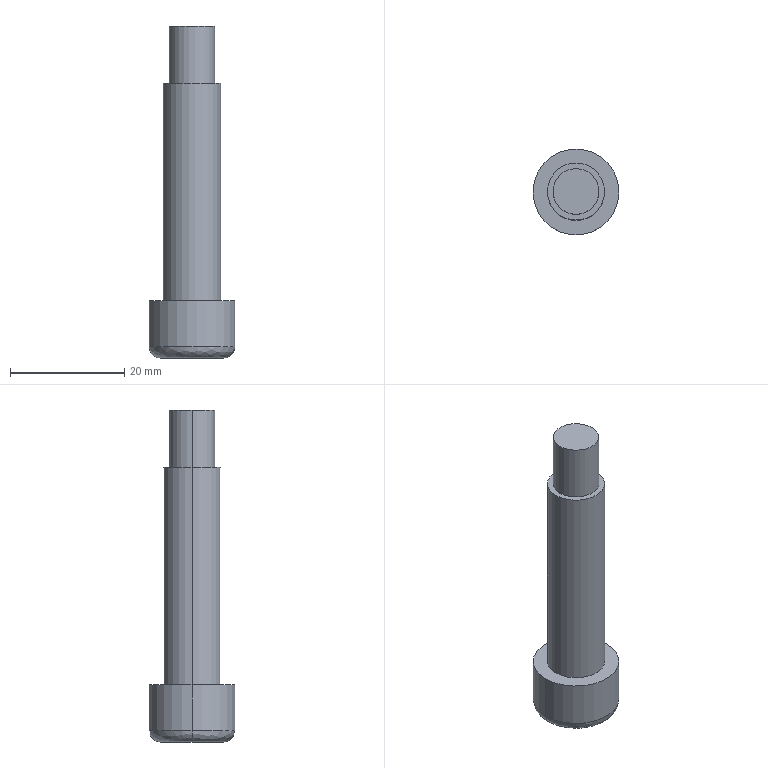Part | STEP file | BULONG BAC M8X10X38 | 1 solid | 19 faces | box 15 x 15 x 58 mm | volume 4939 mm3 | plane 11 | cylinder 6 | spline 2 | commonest cylinder face diameters 8 x2 10 x2 15 x2
STEP:
#1=CARTESIAN_POINT('',(0.,0.,0.));
#2=DIRECTION('',(0.,0.,1.));
#3=DIRECTION('',(1.,0.,0.));
#4=AXIS2_PLACEMENT_3D('',#1,#2,#3);
#5=CARTESIAN_POINT('',(-5.5,0.,0.));
#6=VERTEX_POINT('',#5);
#7=CARTESIAN_POINT('',(5.5,0.,0.));
#8=VERTEX_POINT('',#7);
#9=CARTESIAN_POINT('',(-5.5,0.,0.));
#10=CARTESIAN_POINT('',(-5.5,-11.,0.));
#11=CARTESIAN_POINT('',(5.5,-11.,0.));
#12=CARTESIAN_POINT('',(5.5,0.,0.));
#13=(BOUNDED_CURVE()B_SPLINE_CURVE(3,(#9,#10,#11,#12),.UNSPECIFIED.,.F.,.F.)B_SPLINE_CURVE_WITH_KNOTS((4,4),(0.5,1.),.PIECEWISE_BEZIER_KNOTS.)CURVE()GEOMETRIC_REPRESENTATION_ITEM()RATIONAL_B_SPLINE_CURVE((1.,0.3333,0.3333,1.))REPRESENTATION_ITEM(''));
#14=CARTESIAN_POINT('',(5.5,0.,0.));
#15=CARTESIAN_POINT('',(5.5,-11.,0.));
#16=CARTESIAN_POINT('',(-5.5,-11.,0.));
#17=CARTESIAN_POINT('',(-5.5,0.,0.));
#18=CARTESIAN_POINT('',(6.672,0.,0.));
#19=CARTESIAN_POINT('',(6.672,-13.343,0.));
#20=CARTESIAN_POINT('',(-6.672,-13.343,0.));
#21=CARTESIAN_POINT('',(-6.672,0.,0.));
#22=CARTESIAN_POINT('',(7.5,0.,0.8284));
#23=CARTESIAN_POINT('',(7.5,-15.,0.8284));
#24=CARTESIAN_POINT('',(-7.5,-15.,0.8284));
#25=CARTESIAN_POINT('',(-7.5,0.,0.8284));
#26=CARTESIAN_POINT('',(7.5,0.,2.));
#27=CARTESIAN_POINT('',(7.5,-15.,2.));
#28=CARTESIAN_POINT('',(-7.5,-15.,2.));
#29=CARTESIAN_POINT('',(-7.5,0.,2.));
#30=(BOUNDED_SURFACE()B_SPLINE_SURFACE(3,3,((#14,#15,#16,#17),(#18,#19,#20,#21),(#22,#23,#24,#25),(#26,#27,#28,#29)),.UNSPECIFIED.,.F.,.F.,.F.)B_SPLINE_SURFACE_WITH_KNOTS((4,4),(4,4),(0.,1.),(0.,1.),.PIECEWISE_BEZIER_KNOTS.)GEOMETRIC_REPRESENTATION_ITEM()RATIONAL_B_SPLINE_SURFACE(((1.,0.3333,0.3333,1.),(0.8047,0.2682,0.2682,0.8047),(0.8047,0.2682,0.2682,0.8047),(1.,0.3333,0.3333,1.)))REPRESENTATION_ITEM('')SURFACE());
#31=CARTESIAN_POINT('',(0.,1.));
#32=CARTESIAN_POINT('',(0.,0.));
#33=B_SPLINE_CURVE_WITH_KNOTS('',1,(#31,#32),.UNSPECIFIED.,.F.,.F.,(2,2),(0.5,1.),.PIECEWISE_BEZIER_KNOTS.);
#34=(GEOMETRIC_REPRESENTATION_CONTEXT(2)PARAMETRIC_REPRESENTATION_CONTEXT()REPRESENTATION_CONTEXT('',''));
#35=DEFINITIONAL_REPRESENTATION('',(#33),#34);
#36=PCURVE('',#30,#35);
#37=CARTESIAN_POINT('',(0.,0.,0.));
#38=DIRECTION('',(0.,0.,-1.));
#39=DIRECTION('',(-1.,0.,0.));
#40=AXIS2_PLACEMENT_3D('',#37,#38,#39);
#41=PLANE('',#40);
#42=CARTESIAN_POINT('',(5.5,0.));
#43=CARTESIAN_POINT('',(5.5,-11.));
#44=CARTESIAN_POINT('',(-5.5,-11.));
#45=CARTESIAN_POINT('',(-5.5,0.));
#46=(BOUNDED_CURVE()B_SPLINE_CURVE(3,(#42,#43,#44,#45),.UNSPECIFIED.,.F.,.F.)B_SPLINE_CURVE_WITH_KNOTS((4,4),(0.5,1.),.PIECEWISE_BEZIER_KNOTS.)CURVE()GEOMETRIC_REPRESENTATION_ITEM()RATIONAL_B_SPLINE_CURVE((1.,0.3333,0.3333,1.))REPRESENTATION_ITEM(''));
#47=(GEOMETRIC_REPRESENTATION_CONTEXT(2)PARAMETRIC_REPRESENTATION_CONTEXT()REPRESENTATION_CONTEXT('',''));
#48=DEFINITIONAL_REPRESENTATION('',(#46),#47);
#49=PCURVE('',#41,#48);
#50=SURFACE_CURVE('',#13,(#36,#49),.PCURVE_S1.);
#51=EDGE_CURVE('',#6,#8,#50,.T.);
#52=ORIENTED_EDGE('',*,*,#51,.T.);
#53=CARTESIAN_POINT('',(7.5,0.,2.));
#54=VERTEX_POINT('',#53);
#55=CARTESIAN_POINT('',(5.5,0.,2.));
#56=DIRECTION('',(0.,-1.,0.));
#57=DIRECTION('',(1.,0.,0.));
#58=AXIS2_PLACEMENT_3D('',#55,#56,#57);
#59=CIRCLE('',#58,2.);
#60=CARTESIAN_POINT('',(0.,0.));
#61=CARTESIAN_POINT('',(0.01683,0.));
#62=CARTESIAN_POINT('',(0.04999,0.));
#63=CARTESIAN_POINT('',(0.09843,0.));
#64=CARTESIAN_POINT('',(0.1457,0.));
#65=CARTESIAN_POINT('',(0.192,0.));
#66=CARTESIAN_POINT('',(0.2375,0.));
#67=CARTESIAN_POINT('',(0.2823,0.));
#68=CARTESIAN_POINT('',(0.3265,0.));
#69=CARTESIAN_POINT('',(0.3703,0.));
#70=CARTESIAN_POINT('',(0.4137,0.));
#71=CARTESIAN_POINT('',(0.4569,0.));
#72=CARTESIAN_POINT('',(0.5,0.));
#73=CARTESIAN_POINT('',(0.5431,0.));
#74=CARTESIAN_POINT('',(0.5863,0.));
#75=CARTESIAN_POINT('',(0.6297,0.));
#76=CARTESIAN_POINT('',(0.6735,0.));
#77=CARTESIAN_POINT('',(0.7177,0.));
#78=CARTESIAN_POINT('',(0.7625,0.));
#79=CARTESIAN_POINT('',(0.808,0.));
#80=CARTESIAN_POINT('',(0.8543,0.));
#81=CARTESIAN_POINT('',(0.9016,0.));
#82=CARTESIAN_POINT('',(0.95,0.));
#83=CARTESIAN_POINT('',(0.9832,0.));
#84=CARTESIAN_POINT('',(1.,0.));
#85=B_SPLINE_CURVE_WITH_KNOTS('',3,(#60,#61,#62,#63,#64,#65,#66,#67,#68,#69,#70,#71,#72,#73,#74,#75,#76,#77,#78,#79,#80,#81,#82,#83,#84),.UNSPECIFIED.,.F.,.F.,(4,1,1,1,1,1,1,1,1,1,1,1,1,1,1,1,1,1,1,1,1,1,4),(4.712,4.784,4.855,4.927,4.998,5.069,5.141,5.212,5.284,5.355,5.426,5.498,5.569,5.641,5.712,5.783,5.855,5.926,5.998,6.069,6.14,6.212,6.283),.QUASI_UNIFORM_KNOTS.);
#86=(GEOMETRIC_REPRESENTATION_CONTEXT(2)PARAMETRIC_REPRESENTATION_CONTEXT()REPRESENTATION_CONTEXT('',''));
#87=DEFINITIONAL_REPRESENTATION('',(#85),#86);
#88=PCURVE('',#30,#87);
#89=CARTESIAN_POINT('',(-5.5,0.,0.));
#90=CARTESIAN_POINT('',(-5.5,11.,0.));
#91=CARTESIAN_POINT('',(5.5,11.,0.));
#92=CARTESIAN_POINT('',(5.5,0.,0.));
#93=CARTESIAN_POINT('',(-6.672,0.,0.));
#94=CARTESIAN_POINT('',(-6.672,13.343,0.));
#95=CARTESIAN_POINT('',(6.672,13.343,0.));
#96=CARTESIAN_POINT('',(6.672,0.,0.));
#97=CARTESIAN_POINT('',(-7.5,0.,0.8284));
#98=CARTESIAN_POINT('',(-7.5,15.,0.8284));
#99=CARTESIAN_POINT('',(7.5,15.,0.8284));
#100=CARTESIAN_POINT('',(7.5,0.,0.8284));
#101=CARTESIAN_POINT('',(-7.5,0.,2.));
#102=CARTESIAN_POINT('',(-7.5,15.,2.));
#103=CARTESIAN_POINT('',(7.5,15.,2.));
#104=CARTESIAN_POINT('',(7.5,0.,2.));
#105=(BOUNDED_SURFACE()B_SPLINE_SURFACE(3,3,((#89,#90,#91,#92),(#93,#94,#95,#96),(#97,#98,#99,#100),(#101,#102,#103,#104)),.UNSPECIFIED.,.F.,.F.,.F.)B_SPLINE_SURFACE_WITH_KNOTS((4,4),(4,4),(0.,1.),(0.,1.),.PIECEWISE_BEZIER_KNOTS.)GEOMETRIC_REPRESENTATION_ITEM()RATIONAL_B_SPLINE_SURFACE(((1.,0.3333,0.3333,1.),(0.8047,0.2682,0.2682,0.8047),(0.8047,0.2682,0.2682,0.8047),(1.,0.3333,0.3333,1.)))REPRESENTATION_ITEM('')SURFACE());
#106=CARTESIAN_POINT('',(0.,1.));
#107=CARTESIAN_POINT('',(0.01683,1.));
#108=CARTESIAN_POINT('',(0.04999,1.));
#109=CARTESIAN_POINT('',(0.09843,1.));
#110=CARTESIAN_POINT('',(0.1457,1.));
#111=CARTESIAN_POINT('',(0.192,1.));
#112=CARTESIAN_POINT('',(0.2375,1.));
#113=CARTESIAN_POINT('',(0.2823,1.));
#114=CARTESIAN_POINT('',(0.3265,1.));
#115=CARTESIAN_POINT('',(0.3703,1.));
#116=CARTESIAN_POINT('',(0.4137,1.));
#117=CARTESIAN_POINT('',(0.4569,1.));
#118=CARTESIAN_POINT('',(0.5,1.));
#119=CARTESIAN_POINT('',(0.5431,1.));
#120=CARTESIAN_POINT('',(0.5863,1.));
#121=CARTESIAN_POINT('',(0.6297,1.));
#122=CARTESIAN_POINT('',(0.6735,1.));
#123=CARTESIAN_POINT('',(0.7177,1.));
#124=CARTESIAN_POINT('',(0.7625,1.));
#125=CARTESIAN_POINT('',(0.808,1.));
#126=CARTESIAN_POINT('',(0.8543,1.));
#127=CARTESIAN_POINT('',(0.9016,1.));
#128=CARTESIAN_POINT('',(0.95,1.));
#129=CARTESIAN_POINT('',(0.9832,1.));
#130=CARTESIAN_POINT('',(1.,1.));
#131=B_SPLINE_CURVE_WITH_KNOTS('',3,(#106,#107,#108,#109,#110,#111,#112,#113,#114,#115,#116,#117,#118,#119,#120,#121,#122,#123,#124,#125,#126,#127,#128,#129,#130),.UNSPECIFIED.,.F.,.F.,(4,1,1,1,1,1,1,1,1,1,1,1,1,1,1,1,1,1,1,1,1,1,4),(4.712,4.784,4.855,4.927,4.998,5.069,5.141,5.212,5.284,5.355,5.426,5.498,5.569,5.641,5.712,5.783,5.855,5.926,5.998,6.069,6.14,6.212,6.283),.QUASI_UNIFORM_KNOTS.);
#132=(GEOMETRIC_REPRESENTATION_CONTEXT(2)PARAMETRIC_REPRESENTATION_CONTEXT()REPRESENTATION_CONTEXT('',''));
#133=DEFINITIONAL_REPRESENTATION('',(#131),#132);
#134=PCURVE('',#105,#133);
#135=SURFACE_CURVE('',#59,(#88,#134),.PCURVE_S1.);
#136=EDGE_CURVE('',#8,#54,#135,.T.);
#137=ORIENTED_EDGE('',*,*,#136,.T.);
#138=CARTESIAN_POINT('',(-7.5,0.,2.));
#139=VERTEX_POINT('',#138);
#140=CARTESIAN_POINT('',(0.,0.,2.));
#141=DIRECTION('',(0.,0.,1.));
#142=DIRECTION('',(1.,0.,0.));
#143=AXIS2_PLACEMENT_3D('',#140,#141,#142);
#144=CIRCLE('',#143,7.5);
#145=CARTESIAN_POINT('',(1.,1.));
#146=CARTESIAN_POINT('',(1.,0.9763));
#147=CARTESIAN_POINT('',(1.,0.9319));
#148=CARTESIAN_POINT('',(1.,0.8733));
#149=CARTESIAN_POINT('',(1.,0.8206));
#150=CARTESIAN_POINT('',(1.,0.7724));
#151=CARTESIAN_POINT('',(1.,0.7279));
#152=CARTESIAN_POINT('',(1.,0.6861));
#153=CARTESIAN_POINT('',(1.,0.6465));
#154=CARTESIAN_POINT('',(1.,0.6086));
#155=CARTESIAN_POINT('',(1.,0.5718));
#156=CARTESIAN_POINT('',(1.,0.5357));
#157=CARTESIAN_POINT('',(1.,0.5));
#158=CARTESIAN_POINT('',(1.,0.4643));
#159=CARTESIAN_POINT('',(1.,0.4282));
#160=CARTESIAN_POINT('',(1.,0.3914));
#161=CARTESIAN_POINT('',(1.,0.3535));
#162=CARTESIAN_POINT('',(1.,0.3139));
#163=CARTESIAN_POINT('',(1.,0.2721));
#164=CARTESIAN_POINT('',(1.,0.2276));
#165=CARTESIAN_POINT('',(1.,0.1794));
#166=CARTESIAN_POINT('',(1.,0.1267));
#167=CARTESIAN_POINT('',(1.,0.06805));
#168=CARTESIAN_POINT('',(1.,0.02375));
#169=CARTESIAN_POINT('',(1.,0.));
#170=B_SPLINE_CURVE_WITH_KNOTS('',3,(#145,#146,#147,#148,#149,#150,#151,#152,#153,#154,#155,#156,#157,#158,#159,#160,#161,#162,#163,#164,#165,#166,#167,#168,#169),.UNSPECIFIED.,.F.,.F.,(4,1,1,1,1,1,1,1,1,1,1,1,1,1,1,1,1,1,1,1,1,1,4),(3.142,3.284,3.427,3.57,3.713,3.856,3.998,4.141,4.284,4.427,4.57,4.712,4.855,4.998,5.141,5.284,5.426,5.569,5.712,5.855,5.998,6.14,6.283),.QUASI_UNIFORM_KNOTS.);
#171=(GEOMETRIC_REPRESENTATION_CONTEXT(2)PARAMETRIC_REPRESENTATION_CONTEXT()REPRESENTATION_CONTEXT('',''));
#172=DEFINITIONAL_REPRESENTATION('',(#170),#171);
#173=PCURVE('',#30,#172);
#174=CARTESIAN_POINT('',(0.,0.,0.));
#175=DIRECTION('',(0.,0.,1.));
#176=DIRECTION('',(1.,0.,0.));
#177=AXIS2_PLACEMENT_3D('',#174,#175,#176);
#178=CYLINDRICAL_SURFACE('',#177,7.5);
#179=CARTESIAN_POINT('',(0.,2.));
#180=DIRECTION('',(1.,0.));
#181=VECTOR('',#180,1.);
#182=LINE('',#179,#181);
#183=(GEOMETRIC_REPRESENTATION_CONTEXT(2)PARAMETRIC_REPRESENTATION_CONTEXT()REPRESENTATION_CONTEXT('',''));
#184=DEFINITIONAL_REPRESENTATION('',(#182),#183);
#185=PCURVE('',#178,#184);
#186=SURFACE_CURVE('',#144,(#173,#185),.PCURVE_S1.);
#187=EDGE_CURVE('',#139,#54,#186,.T.);
#188=ORIENTED_EDGE('',*,*,#187,.F.);
#189=CARTESIAN_POINT('',(-5.5,0.,2.));
#190=DIRECTION('',(0.,1.,0.));
#191=DIRECTION('',(-1.,0.,0.));
#192=AXIS2_PLACEMENT_3D('',#189,#190,#191);
#193=CIRCLE('',#192,2.);
#194=CARTESIAN_POINT('',(0.,1.));
#195=CARTESIAN_POINT('',(0.01683,1.));
#196=CARTESIAN_POINT('',(0.04999,1.));
#197=CARTESIAN_POINT('',(0.09843,1.));
#198=CARTESIAN_POINT('',(0.1457,1.));
#199=CARTESIAN_POINT('',(0.192,1.));
#200=CARTESIAN_POINT('',(0.2375,1.));
#201=CARTESIAN_POINT('',(0.2823,1.));
#202=CARTESIAN_POINT('',(0.3265,1.));
#203=CARTESIAN_POINT('',(0.3703,1.));
#204=CARTESIAN_POINT('',(0.4137,1.));
#205=CARTESIAN_POINT('',(0.4569,1.));
#206=CARTESIAN_POINT('',(0.5,1.));
#207=CARTESIAN_POINT('',(0.5431,1.));
#208=CARTESIAN_POINT('',(0.5863,1.));
#209=CARTESIAN_POINT('',(0.6297,1.));
#210=CARTESIAN_POINT('',(0.6735,1.));
#211=CARTESIAN_POINT('',(0.7177,1.));
#212=CARTESIAN_POINT('',(0.7625,1.));
#213=CARTESIAN_POINT('',(0.808,1.));
#214=CARTESIAN_POINT('',(0.8543,1.));
#215=CARTESIAN_POINT('',(0.9016,1.));
#216=CARTESIAN_POINT('',(0.95,1.));
#217=CARTESIAN_POINT('',(0.9832,1.));
#218=CARTESIAN_POINT('',(1.,1.));
#219=B_SPLINE_CURVE_WITH_KNOTS('',3,(#194,#195,#196,#197,#198,#199,#200,#201,#202,#203,#204,#205,#206,#207,#208,#209,#210,#211,#212,#213,#214,#215,#216,#217,#218),.UNSPECIFIED.,.F.,.F.,(4,1,1,1,1,1,1,1,1,1,1,1,1,1,1,1,1,1,1,1,1,1,4),(4.712,4.784,4.855,4.927,4.998,5.069,5.141,5.212,5.284,5.355,5.426,5.498,5.569,5.641,5.712,5.783,5.855,5.926,5.998,6.069,6.14,6.212,6.283),.QUASI_UNIFORM_KNOTS.);
#220=(GEOMETRIC_REPRESENTATION_CONTEXT(2)PARAMETRIC_REPRESENTATION_CONTEXT()REPRESENTATION_CONTEXT('',''));
#221=DEFINITIONAL_REPRESENTATION('',(#219),#220);
#222=PCURVE('',#30,#221);
#223=CARTESIAN_POINT('',(0.,0.));
#224=CARTESIAN_POINT('',(0.01683,0.));
#225=CARTESIAN_POINT('',(0.04999,0.));
#226=CARTESIAN_POINT('',(0.09843,0.));
#227=CARTESIAN_POINT('',(0.1457,0.));
#228=CARTESIAN_POINT('',(0.192,0.));
#229=CARTESIAN_POINT('',(0.2375,0.));
#230=CARTESIAN_POINT('',(0.2823,0.));
#231=CARTESIAN_POINT('',(0.3265,0.));
#232=CARTESIAN_POINT('',(0.3703,0.));
#233=CARTESIAN_POINT('',(0.4137,0.));
#234=CARTESIAN_POINT('',(0.4569,0.));
#235=CARTESIAN_POINT('',(0.5,0.));
#236=CARTESIAN_POINT('',(0.5431,0.));
#237=CARTESIAN_POINT('',(0.5863,0.));
#238=CARTESIAN_POINT('',(0.6297,0.));
#239=CARTESIAN_POINT('',(0.6735,0.));
#240=CARTESIAN_POINT('',(0.7177,0.));
#241=CARTESIAN_POINT('',(0.7625,0.));
#242=CARTESIAN_POINT('',(0.808,0.));
#243=CARTESIAN_POINT('',(0.8543,0.));
#244=CARTESIAN_POINT('',(0.9016,0.));
#245=CARTESIAN_POINT('',(0.95,0.));
#246=CARTESIAN_POINT('',(0.9832,0.));
#247=CARTESIAN_POINT('',(1.,0.));
#248=B_SPLINE_CURVE_WITH_KNOTS('',3,(#223,#224,#225,#226,#227,#228,#229,#230,#231,#232,#233,#234,#235,#236,#237,#238,#239,#240,#241,#242,#243,#244,#245,#246,#247),.UNSPECIFIED.,.F.,.F.,(4,1,1,1,1,1,1,1,1,1,1,1,1,1,1,1,1,1,1,1,1,1,4),(4.712,4.784,4.855,4.927,4.998,5.069,5.141,5.212,5.284,5.355,5.426,5.498,5.569,5.641,5.712,5.783,5.855,5.926,5.998,6.069,6.14,6.212,6.283),.QUASI_UNIFORM_KNOTS.);
#249=(GEOMETRIC_REPRESENTATION_CONTEXT(2)PARAMETRIC_REPRESENTATION_CONTEXT()REPRESENTATION_CONTEXT('',''));
#250=DEFINITIONAL_REPRESENTATION('',(#248),#249);
#251=PCURVE('',#105,#250);
#252=SURFACE_CURVE('',#193,(#222,#251),.PCURVE_S1.);
#253=EDGE_CURVE('',#6,#139,#252,.T.);
#254=ORIENTED_EDGE('',*,*,#253,.F.);
#255=EDGE_LOOP('',(#52,#137,#188,#254));
#256=FACE_BOUND('',#255,.T.);
#257=ADVANCED_FACE('',(#256),#30,.T.);
#258=CARTESIAN_POINT('',(5.,0.,10.));
#259=VERTEX_POINT('',#258);
#260=CARTESIAN_POINT('',(-5.,0.,10.));
#261=VERTEX_POINT('',#260);
#262=CARTESIAN_POINT('',(0.,0.,10.));
#263=DIRECTION('',(0.,0.,1.));
#264=DIRECTION('',(1.,0.,0.));
#265=AXIS2_PLACEMENT_3D('',#262,#263,#264);
#266=CIRCLE('',#265,5.);
#267=CARTESIAN_POINT('',(0.,0.,10.));
#268=DIRECTION('',(0.,0.,1.));
#269=DIRECTION('',(1.,0.,0.));
#270=AXIS2_PLACEMENT_3D('',#267,#268,#269);
#271=CYLINDRICAL_SURFACE('',#270,5.);
#272=CARTESIAN_POINT('',(0.,0.));
#273=DIRECTION('',(1.,0.));
#274=VECTOR('',#273,1.);
#275=LINE('',#272,#274);
#276=(GEOMETRIC_REPRESENTATION_CONTEXT(2)PARAMETRIC_REPRESENTATION_CONTEXT()REPRESENTATION_CONTEXT('',''));
#277=DEFINITIONAL_REPRESENTATION('',(#275),#276);
#278=PCURVE('',#271,#277);
#279=CARTESIAN_POINT('',(0.,0.,10.));
#280=DIRECTION('',(0.,0.,-1.));
#281=DIRECTION('',(-1.,0.,0.));
#282=AXIS2_PLACEMENT_3D('',#279,#280,#281);
#283=PLANE('',#282);
#284=CARTESIAN_POINT('',(-5.,0.));
#285=CARTESIAN_POINT('',(-5.,8.66));
#286=CARTESIAN_POINT('',(2.5,4.33));
#287=CARTESIAN_POINT('',(10.,0.));
#288=CARTESIAN_POINT('',(2.5,-4.33));
#289=CARTESIAN_POINT('',(-5.,-8.66));
#290=CARTESIAN_POINT('',(-5.,0.));
#291=(BOUNDED_CURVE()B_SPLINE_CURVE(2,(#284,#285,#286,#287,#288,#289,#290),.UNSPECIFIED.,.T.,.F.)B_SPLINE_CURVE_WITH_KNOTS((1,2,2,2,2,1),(-2.094,0.,2.094,4.189,6.283,8.378),.UNSPECIFIED.)CURVE()GEOMETRIC_REPRESENTATION_ITEM()RATIONAL_B_SPLINE_CURVE((1.,0.5,1.,0.5,1.,0.5,1.))REPRESENTATION_ITEM(''));
#292=(GEOMETRIC_REPRESENTATION_CONTEXT(2)PARAMETRIC_REPRESENTATION_CONTEXT()REPRESENTATION_CONTEXT('',''));
#293=DEFINITIONAL_REPRESENTATION('',(#291),#292);
#294=PCURVE('',#283,#293);
#295=SURFACE_CURVE('',#266,(#278,#294),.PCURVE_S1.);
#296=EDGE_CURVE('',#259,#261,#295,.T.);
#297=ORIENTED_EDGE('',*,*,#296,.T.);
#298=CARTESIAN_POINT('',(-5.,0.,48.));
#299=VERTEX_POINT('',#298);
#300=CARTESIAN_POINT('',(-5.,0.,10.));
#301=DIRECTION('',(0.,0.,1.));
#302=VECTOR('',#301,1.);
#303=LINE('',#300,#302);
#304=CARTESIAN_POINT('',(3.142,0.));
#305=DIRECTION('',(0.,1.));
#306=VECTOR('',#305,1.);
#307=LINE('',#304,#306);
#308=(GEOMETRIC_REPRESENTATION_CONTEXT(2)PARAMETRIC_REPRESENTATION_CONTEXT()REPRESENTATION_CONTEXT('',''));
#309=DEFINITIONAL_REPRESENTATION('',(#307),#308);
#310=PCURVE('',#271,#309);
#311=CARTESIAN_POINT('',(0.,0.,10.));
#312=DIRECTION('',(0.,0.,1.));
#313=DIRECTION('',(1.,0.,0.));
#314=AXIS2_PLACEMENT_3D('',#311,#312,#313);
#315=CYLINDRICAL_SURFACE('',#314,5.);
#316=CARTESIAN_POINT('',(3.142,0.));
#317=DIRECTION('',(0.,1.));
#318=VECTOR('',#317,1.);
#319=LINE('',#316,#318);
#320=(GEOMETRIC_REPRESENTATION_CONTEXT(2)PARAMETRIC_REPRESENTATION_CONTEXT()REPRESENTATION_CONTEXT('',''));
#321=DEFINITIONAL_REPRESENTATION('',(#319),#320);
#322=PCURVE('',#315,#321);
#323=SURFACE_CURVE('',#303,(#310,#322),.PCURVE_S1.);
#324=EDGE_CURVE('',#261,#299,#323,.T.);
#325=ORIENTED_EDGE('',*,*,#324,.T.);
#326=CARTESIAN_POINT('',(5.,0.,48.));
#327=VERTEX_POINT('',#326);
#328=CARTESIAN_POINT('',(0.,0.,48.));
#329=DIRECTION('',(0.,0.,-1.));
#330=DIRECTION('',(1.,0.,0.));
#331=AXIS2_PLACEMENT_3D('',#328,#329,#330);
#332=CIRCLE('',#331,5.);
#333=CARTESIAN_POINT('',(6.283,38.));
#334=DIRECTION('',(-1.,0.));
#335=VECTOR('',#334,1.);
#336=LINE('',#333,#335);
#337=(GEOMETRIC_REPRESENTATION_CONTEXT(2)PARAMETRIC_REPRESENTATION_CONTEXT()REPRESENTATION_CONTEXT('',''));
#338=DEFINITIONAL_REPRESENTATION('',(#336),#337);
#339=PCURVE('',#271,#338);
#340=CARTESIAN_POINT('',(0.,0.,48.));
#341=DIRECTION('',(0.,0.,-1.));
#342=DIRECTION('',(-1.,0.,0.));
#343=AXIS2_PLACEMENT_3D('',#340,#341,#342);
#344=PLANE('',#343);
#345=CARTESIAN_POINT('',(0.,0.));
#346=DIRECTION('',(-1.,0.));
#347=AXIS2_PLACEMENT_2D('',#345,#346);
#348=CIRCLE('',#347,5.);
#349=(GEOMETRIC_REPRESENTATION_CONTEXT(2)PARAMETRIC_REPRESENTATION_CONTEXT()REPRESENTATION_CONTEXT('',''));
#350=DEFINITIONAL_REPRESENTATION('',(#348),#349);
#351=PCURVE('',#344,#350);
#352=SURFACE_CURVE('',#332,(#339,#351),.PCURVE_S1.);
#353=EDGE_CURVE('',#299,#327,#352,.T.);
#354=ORIENTED_EDGE('',*,*,#353,.T.);
#355=CARTESIAN_POINT('',(5.,0.,10.));
#356=DIRECTION('',(0.,0.,1.));
#357=VECTOR('',#356,1.);
#358=LINE('',#355,#357);
#359=CARTESIAN_POINT('',(0.,0.));
#360=DIRECTION('',(0.,1.));
#361=VECTOR('',#360,1.);
#362=LINE('',#359,#361);
#363=(GEOMETRIC_REPRESENTATION_CONTEXT(2)PARAMETRIC_REPRESENTATION_CONTEXT()REPRESENTATION_CONTEXT('',''));
#364=DEFINITIONAL_REPRESENTATION('',(#362),#363);
#365=PCURVE('',#271,#364);
#366=CARTESIAN_POINT('',(6.283,0.));
#367=DIRECTION('',(0.,1.));
#368=VECTOR('',#367,1.);
#369=LINE('',#366,#368);
#370=(GEOMETRIC_REPRESENTATION_CONTEXT(2)PARAMETRIC_REPRESENTATION_CONTEXT()REPRESENTATION_CONTEXT('',''));
#371=DEFINITIONAL_REPRESENTATION('',(#369),#370);
#372=PCURVE('',#315,#371);
#373=SURFACE_CURVE('',#358,(#365,#372),.PCURVE_S1.);
#374=EDGE_CURVE('',#259,#327,#373,.T.);
#375=ORIENTED_EDGE('',*,*,#374,.F.);
#376=EDGE_LOOP('',(#297,#325,#354,#375));
#377=FACE_BOUND('',#376,.T.);
#378=ADVANCED_FACE('',(#377),#271,.T.);
#379=CARTESIAN_POINT('',(0.,0.,2.));
#380=DIRECTION('',(0.,0.,1.));
#381=DIRECTION('',(1.,0.,0.));
#382=AXIS2_PLACEMENT_3D('',#379,#380,#381);
#383=CIRCLE('',#382,7.5);
#384=CARTESIAN_POINT('',(0.,0.,0.));
#385=DIRECTION('',(0.,0.,1.));
#386=DIRECTION('',(1.,0.,0.));
#387=AXIS2_PLACEMENT_3D('',#384,#385,#386);
#388=CYLINDRICAL_SURFACE('',#387,7.5);
#389=CARTESIAN_POINT('',(0.,2.));
#390=DIRECTION('',(1.,0.));
#391=VECTOR('',#390,1.);
#392=LINE('',#389,#391);
#393=(GEOMETRIC_REPRESENTATION_CONTEXT(2)PARAMETRIC_REPRESENTATION_CONTEXT()REPRESENTATION_CONTEXT('',''));
#394=DEFINITIONAL_REPRESENTATION('',(#392),#393);
#395=PCURVE('',#388,#394);
#396=CARTESIAN_POINT('',(1.,1.));
#397=CARTESIAN_POINT('',(1.,0.9763));
#398=CARTESIAN_POINT('',(1.,0.9319));
#399=CARTESIAN_POINT('',(1.,0.8733));
#400=CARTESIAN_POINT('',(1.,0.8206));
#401=CARTESIAN_POINT('',(1.,0.7724));
#402=CARTESIAN_POINT('',(1.,0.7279));
#403=CARTESIAN_POINT('',(1.,0.6861));
#404=CARTESIAN_POINT('',(1.,0.6465));
#405=CARTESIAN_POINT('',(1.,0.6086));
#406=CARTESIAN_POINT('',(1.,0.5718));
#407=CARTESIAN_POINT('',(1.,0.5357));
#408=CARTESIAN_POINT('',(1.,0.5));
#409=CARTESIAN_POINT('',(1.,0.4643));
#410=CARTESIAN_POINT('',(1.,0.4282));
#411=CARTESIAN_POINT('',(1.,0.3914));
#412=CARTESIAN_POINT('',(1.,0.3535));
#413=CARTESIAN_POINT('',(1.,0.3139));
#414=CARTESIAN_POINT('',(1.,0.2721));
#415=CARTESIAN_POINT('',(1.,0.2276));
#416=CARTESIAN_POINT('',(1.,0.1794));
#417=CARTESIAN_POINT('',(1.,0.1267));
#418=CARTESIAN_POINT('',(1.,0.06805));
#419=CARTESIAN_POINT('',(1.,0.02375));
#420=CARTESIAN_POINT('',(1.,0.));
#421=B_SPLINE_CURVE_WITH_KNOTS('',3,(#396,#397,#398,#399,#400,#401,#402,#403,#404,#405,#406,#407,#408,#409,#410,#411,#412,#413,#414,#415,#416,#417,#418,#419,#420),.UNSPECIFIED.,.F.,.F.,(4,1,1,1,1,1,1,1,1,1,1,1,1,1,1,1,1,1,1,1,1,1,4),(0.,0.1428,0.2856,0.4284,0.5712,0.714,0.8568,0.9996,1.142,1.285,1.428,1.571,1.714,1.856,1.999,2.142,2.285,2.428,2.57,2.713,2.856,2.999,3.142),.QUASI_UNIFORM_KNOTS.);
#422=(GEOMETRIC_REPRESENTATION_CONTEXT(2)PARAMETRIC_REPRESENTATION_CONTEXT()REPRESENTATION_CONTEXT('',''));
#423=DEFINITIONAL_REPRESENTATION('',(#421),#422);
#424=PCURVE('',#105,#423);
#425=SURFACE_CURVE('',#383,(#395,#424),.PCURVE_S1.);
#426=EDGE_CURVE('',#54,#139,#425,.T.);
#427=ORIENTED_EDGE('',*,*,#426,.T.);
#428=CARTESIAN_POINT('',(-7.5,0.,10.));
#429=VERTEX_POINT('',#428);
#430=CARTESIAN_POINT('',(-7.5,0.,0.));
#431=DIRECTION('',(0.,0.,1.));
#432=VECTOR('',#431,1.);
#433=LINE('',#430,#432);
#434=CARTESIAN_POINT('',(3.142,0.));
#435=DIRECTION('',(0.,1.));
#436=VECTOR('',#435,1.);
#437=LINE('',#434,#436);
#438=(GEOMETRIC_REPRESENTATION_CONTEXT(2)PARAMETRIC_REPRESENTATION_CONTEXT()REPRESENTATION_CONTEXT('',''));
#439=DEFINITIONAL_REPRESENTATION('',(#437),#438);
#440=PCURVE('',#388,#439);
#441=CARTESIAN_POINT('',(3.142,0.));
#442=DIRECTION('',(0.,1.));
#443=VECTOR('',#442,1.);
#444=LINE('',#441,#443);
#445=(GEOMETRIC_REPRESENTATION_CONTEXT(2)PARAMETRIC_REPRESENTATION_CONTEXT()REPRESENTATION_CONTEXT('',''));
#446=DEFINITIONAL_REPRESENTATION('',(#444),#445);
#447=PCURVE('',#178,#446);
#448=SURFACE_CURVE('',#433,(#440,#447),.PCURVE_S1.);
#449=EDGE_CURVE('',#139,#429,#448,.T.);
#450=ORIENTED_EDGE('',*,*,#449,.T.);
#451=CARTESIAN_POINT('',(7.5,0.,10.));
#452=VERTEX_POINT('',#451);
#453=CARTESIAN_POINT('',(0.,0.,10.));
#454=DIRECTION('',(0.,0.,-1.));
#455=DIRECTION('',(1.,0.,0.));
#456=AXIS2_PLACEMENT_3D('',#453,#454,#455);
#457=CIRCLE('',#456,7.5);
#458=CARTESIAN_POINT('',(6.283,10.));
#459=DIRECTION('',(-1.,0.));
#460=VECTOR('',#459,1.);
#461=LINE('',#458,#460);
#462=(GEOMETRIC_REPRESENTATION_CONTEXT(2)PARAMETRIC_REPRESENTATION_CONTEXT()REPRESENTATION_CONTEXT('',''));
#463=DEFINITIONAL_REPRESENTATION('',(#461),#462);
#464=PCURVE('',#388,#463);
#465=CARTESIAN_POINT('',(0.,0.));
#466=DIRECTION('',(-1.,0.));
#467=AXIS2_PLACEMENT_2D('',#465,#466);
#468=CIRCLE('',#467,7.5);
#469=(GEOMETRIC_REPRESENTATION_CONTEXT(2)PARAMETRIC_REPRESENTATION_CONTEXT()REPRESENTATION_CONTEXT('',''));
#470=DEFINITIONAL_REPRESENTATION('',(#468),#469);
#471=PCURVE('',#283,#470);
#472=SURFACE_CURVE('',#457,(#464,#471),.PCURVE_S1.);
#473=EDGE_CURVE('',#429,#452,#472,.T.);
#474=ORIENTED_EDGE('',*,*,#473,.T.);
#475=CARTESIAN_POINT('',(7.5,0.,0.));
#476=DIRECTION('',(0.,0.,1.));
#477=VECTOR('',#476,1.);
#478=LINE('',#475,#477);
#479=CARTESIAN_POINT('',(0.,0.));
#480=DIRECTION('',(0.,1.));
#481=VECTOR('',#480,1.);
#482=LINE('',#479,#481);
#483=(GEOMETRIC_REPRESENTATION_CONTEXT(2)PARAMETRIC_REPRESENTATION_CONTEXT()REPRESENTATION_CONTEXT('',''));
#484=DEFINITIONAL_REPRESENTATION('',(#482),#483);
#485=PCURVE('',#388,#484);
#486=CARTESIAN_POINT('',(6.283,0.));
#487=DIRECTION('',(0.,1.));
#488=VECTOR('',#487,1.);
#489=LINE('',#486,#488);
#490=(GEOMETRIC_REPRESENTATION_CONTEXT(2)PARAMETRIC_REPRESENTATION_CONTEXT()REPRESENTATION_CONTEXT('',''));
#491=DEFINITIONAL_REPRESENTATION('',(#489),#490);
#492=PCURVE('',#178,#491);
#493=SURFACE_CURVE('',#478,(#485,#492),.PCURVE_S1.);
#494=EDGE_CURVE('',#54,#452,#493,.T.);
#495=ORIENTED_EDGE('',*,*,#494,.F.);
#496=EDGE_LOOP('',(#427,#450,#474,#495));
#497=FACE_BOUND('',#496,.T.);
#498=ADVANCED_FACE('',(#497),#388,.T.);
#499=CARTESIAN_POINT('',(4.,0.,48.));
#500=VERTEX_POINT('',#499);
#501=CARTESIAN_POINT('',(-4.,0.,48.));
#502=VERTEX_POINT('',#501);
#503=CARTESIAN_POINT('',(0.,0.,48.));
#504=DIRECTION('',(0.,0.,1.));
#505=DIRECTION('',(1.,0.,0.));
#506=AXIS2_PLACEMENT_3D('',#503,#504,#505);
#507=CIRCLE('',#506,4.);
#508=CARTESIAN_POINT('',(0.,0.,48.));
#509=DIRECTION('',(0.,0.,1.));
#510=DIRECTION('',(1.,0.,0.));
#511=AXIS2_PLACEMENT_3D('',#508,#509,#510);
#512=CYLINDRICAL_SURFACE('',#511,4.);
#513=CARTESIAN_POINT('',(0.,0.));
#514=DIRECTION('',(1.,0.));
#515=VECTOR('',#514,1.);
#516=LINE('',#513,#515);
#517=(GEOMETRIC_REPRESENTATION_CONTEXT(2)PARAMETRIC_REPRESENTATION_CONTEXT()REPRESENTATION_CONTEXT('',''));
#518=DEFINITIONAL_REPRESENTATION('',(#516),#517);
#519=PCURVE('',#512,#518);
#520=CARTESIAN_POINT('',(-4.,0.));
#521=CARTESIAN_POINT('',(-4.,6.928));
#522=CARTESIAN_POINT('',(2.,3.464));
#523=CARTESIAN_POINT('',(8.,0.));
#524=CARTESIAN_POINT('',(2.,-3.464));
#525=CARTESIAN_POINT('',(-4.,-6.928));
#526=CARTESIAN_POINT('',(-4.,0.));
#527=(BOUNDED_CURVE()B_SPLINE_CURVE(2,(#520,#521,#522,#523,#524,#525,#526),.UNSPECIFIED.,.T.,.F.)B_SPLINE_CURVE_WITH_KNOTS((1,2,2,2,2,1),(-2.094,0.,2.094,4.189,6.283,8.378),.UNSPECIFIED.)CURVE()GEOMETRIC_REPRESENTATION_ITEM()RATIONAL_B_SPLINE_CURVE((1.,0.5,1.,0.5,1.,0.5,1.))REPRESENTATION_ITEM(''));
#528=(GEOMETRIC_REPRESENTATION_CONTEXT(2)PARAMETRIC_REPRESENTATION_CONTEXT()REPRESENTATION_CONTEXT('',''));
#529=DEFINITIONAL_REPRESENTATION('',(#527),#528);
#530=PCURVE('',#344,#529);
#531=SURFACE_CURVE('',#507,(#519,#530),.PCURVE_S1.);
#532=EDGE_CURVE('',#500,#502,#531,.T.);
#533=ORIENTED_EDGE('',*,*,#532,.T.);
#534=CARTESIAN_POINT('',(-4.,0.,58.));
#535=VERTEX_POINT('',#534);
#536=CARTESIAN_POINT('',(-4.,0.,48.));
#537=DIRECTION('',(0.,0.,1.));
#538=VECTOR('',#537,1.);
#539=LINE('',#536,#538);
#540=CARTESIAN_POINT('',(3.142,0.));
#541=DIRECTION('',(0.,1.));
#542=VECTOR('',#541,1.);
#543=LINE('',#540,#542);
#544=(GEOMETRIC_REPRESENTATION_CONTEXT(2)PARAMETRIC_REPRESENTATION_CONTEXT()REPRESENTATION_CONTEXT('',''));
#545=DEFINITIONAL_REPRESENTATION('',(#543),#544);
#546=PCURVE('',#512,#545);
#547=CARTESIAN_POINT('',(0.,0.,48.));
#548=DIRECTION('',(0.,0.,1.));
#549=DIRECTION('',(1.,0.,0.));
#550=AXIS2_PLACEMENT_3D('',#547,#548,#549);
#551=CYLINDRICAL_SURFACE('',#550,4.);
#552=CARTESIAN_POINT('',(3.142,0.));
#553=DIRECTION('',(0.,1.));
#554=VECTOR('',#553,1.);
#555=LINE('',#552,#554);
#556=(GEOMETRIC_REPRESENTATION_CONTEXT(2)PARAMETRIC_REPRESENTATION_CONTEXT()REPRESENTATION_CONTEXT('',''));
#557=DEFINITIONAL_REPRESENTATION('',(#555),#556);
#558=PCURVE('',#551,#557);
#559=SURFACE_CURVE('',#539,(#546,#558),.PCURVE_S1.);
#560=EDGE_CURVE('',#502,#535,#559,.T.);
#561=ORIENTED_EDGE('',*,*,#560,.T.);
#562=CARTESIAN_POINT('',(4.,0.,58.));
#563=VERTEX_POINT('',#562);
#564=CARTESIAN_POINT('',(0.,0.,58.));
#565=DIRECTION('',(0.,0.,-1.));
#566=DIRECTION('',(1.,0.,0.));
#567=AXIS2_PLACEMENT_3D('',#564,#565,#566);
#568=CIRCLE('',#567,4.);
#569=CARTESIAN_POINT('',(6.283,10.));
#570=DIRECTION('',(-1.,0.));
#571=VECTOR('',#570,1.);
#572=LINE('',#569,#571);
#573=(GEOMETRIC_REPRESENTATION_CONTEXT(2)PARAMETRIC_REPRESENTATION_CONTEXT()REPRESENTATION_CONTEXT('',''));
#574=DEFINITIONAL_REPRESENTATION('',(#572),#573);
#575=PCURVE('',#512,#574);
#576=CARTESIAN_POINT('',(0.,0.,58.));
#577=DIRECTION('',(0.,0.,-1.));
#578=DIRECTION('',(-1.,0.,0.));
#579=AXIS2_PLACEMENT_3D('',#576,#577,#578);
#580=PLANE('',#579);
#581=CARTESIAN_POINT('',(0.,0.));
#582=DIRECTION('',(-1.,0.));
#583=AXIS2_PLACEMENT_2D('',#581,#582);
#584=CIRCLE('',#583,4.);
#585=(GEOMETRIC_REPRESENTATION_CONTEXT(2)PARAMETRIC_REPRESENTATION_CONTEXT()REPRESENTATION_CONTEXT('',''));
#586=DEFINITIONAL_REPRESENTATION('',(#584),#585);
#587=PCURVE('',#580,#586);
#588=SURFACE_CURVE('',#568,(#575,#587),.PCURVE_S1.);
#589=EDGE_CURVE('',#535,#563,#588,.T.);
#590=ORIENTED_EDGE('',*,*,#589,.T.);
#591=CARTESIAN_POINT('',(4.,0.,48.));
#592=DIRECTION('',(0.,0.,1.));
#593=VECTOR('',#592,1.);
#594=LINE('',#591,#593);
#595=CARTESIAN_POINT('',(0.,0.));
#596=DIRECTION('',(0.,1.));
#597=VECTOR('',#596,1.);
#598=LINE('',#595,#597);
#599=(GEOMETRIC_REPRESENTATION_CONTEXT(2)PARAMETRIC_REPRESENTATION_CONTEXT()REPRESENTATION_CONTEXT('',''));
#600=DEFINITIONAL_REPRESENTATION('',(#598),#599);
#601=PCURVE('',#512,#600);
#602=CARTESIAN_POINT('',(6.283,0.));
#603=DIRECTION('',(0.,1.));
#604=VECTOR('',#603,1.);
#605=LINE('',#602,#604);
#606=(GEOMETRIC_REPRESENTATION_CONTEXT(2)PARAMETRIC_REPRESENTATION_CONTEXT()REPRESENTATION_CONTEXT('',''));
#607=DEFINITIONAL_REPRESENTATION('',(#605),#606);
#608=PCURVE('',#551,#607);
#609=SURFACE_CURVE('',#594,(#601,#608),.PCURVE_S1.);
#610=EDGE_CURVE('',#500,#563,#609,.T.);
#611=ORIENTED_EDGE('',*,*,#610,.F.);
#612=EDGE_LOOP('',(#533,#561,#590,#611));
#613=FACE_BOUND('',#612,.T.);
#614=ADVANCED_FACE('',(#613),#512,.T.);
#615=ORIENTED_EDGE('',*,*,#324,.F.);
#616=CARTESIAN_POINT('',(0.,0.,10.));
#617=DIRECTION('',(0.,0.,1.));
#618=DIRECTION('',(1.,0.,0.));
#619=AXIS2_PLACEMENT_3D('',#616,#617,#618);
#620=CIRCLE('',#619,5.);
#621=CARTESIAN_POINT('',(0.,0.));
#622=DIRECTION('',(1.,0.));
#623=VECTOR('',#622,1.);
#624=LINE('',#621,#623);
#625=(GEOMETRIC_REPRESENTATION_CONTEXT(2)PARAMETRIC_REPRESENTATION_CONTEXT()REPRESENTATION_CONTEXT('',''));
#626=DEFINITIONAL_REPRESENTATION('',(#624),#625);
#627=PCURVE('',#315,#626);
#628=CARTESIAN_POINT('',(-5.,0.));
#629=CARTESIAN_POINT('',(-5.,8.66));
#630=CARTESIAN_POINT('',(2.5,4.33));
#631=CARTESIAN_POINT('',(10.,0.));
#632=CARTESIAN_POINT('',(2.5,-4.33));
#633=CARTESIAN_POINT('',(-5.,-8.66));
#634=CARTESIAN_POINT('',(-5.,0.));
#635=(BOUNDED_CURVE()B_SPLINE_CURVE(2,(#628,#629,#630,#631,#632,#633,#634),.UNSPECIFIED.,.T.,.F.)B_SPLINE_CURVE_WITH_KNOTS((1,2,2,2,2,1),(-2.094,0.,2.094,4.189,6.283,8.378),.UNSPECIFIED.)CURVE()GEOMETRIC_REPRESENTATION_ITEM()RATIONAL_B_SPLINE_CURVE((1.,0.5,1.,0.5,1.,0.5,1.))REPRESENTATION_ITEM(''));
#636=(GEOMETRIC_REPRESENTATION_CONTEXT(2)PARAMETRIC_REPRESENTATION_CONTEXT()REPRESENTATION_CONTEXT('',''));
#637=DEFINITIONAL_REPRESENTATION('',(#635),#636);
#638=PCURVE('',#283,#637);
#639=SURFACE_CURVE('',#620,(#627,#638),.PCURVE_S1.);
#640=EDGE_CURVE('',#261,#259,#639,.T.);
#641=ORIENTED_EDGE('',*,*,#640,.T.);
#642=ORIENTED_EDGE('',*,*,#374,.T.);
#643=CARTESIAN_POINT('',(0.,0.,48.));
#644=DIRECTION('',(0.,0.,-1.));
#645=DIRECTION('',(1.,0.,0.));
#646=AXIS2_PLACEMENT_3D('',#643,#644,#645);
#647=CIRCLE('',#646,5.);
#648=CARTESIAN_POINT('',(6.283,38.));
#649=DIRECTION('',(-1.,0.));
#650=VECTOR('',#649,1.);
#651=LINE('',#648,#650);
#652=(GEOMETRIC_REPRESENTATION_CONTEXT(2)PARAMETRIC_REPRESENTATION_CONTEXT()REPRESENTATION_CONTEXT('',''));
#653=DEFINITIONAL_REPRESENTATION('',(#651),#652);
#654=PCURVE('',#315,#653);
#655=CARTESIAN_POINT('',(0.,0.));
#656=DIRECTION('',(-1.,0.));
#657=AXIS2_PLACEMENT_2D('',#655,#656);
#658=CIRCLE('',#657,5.);
#659=(GEOMETRIC_REPRESENTATION_CONTEXT(2)PARAMETRIC_REPRESENTATION_CONTEXT()REPRESENTATION_CONTEXT('',''));
#660=DEFINITIONAL_REPRESENTATION('',(#658),#659);
#661=PCURVE('',#344,#660);
#662=SURFACE_CURVE('',#647,(#654,#661),.PCURVE_S1.);
#663=EDGE_CURVE('',#327,#299,#662,.T.);
#664=ORIENTED_EDGE('',*,*,#663,.T.);
#665=EDGE_LOOP('',(#615,#641,#642,#664));
#666=FACE_BOUND('',#665,.T.);
#667=ADVANCED_FACE('',(#666),#315,.T.);
#668=ORIENTED_EDGE('',*,*,#296,.F.);
#669=ORIENTED_EDGE('',*,*,#640,.F.);
#670=EDGE_LOOP('',(#668,#669));
#671=FACE_BOUND('',#670,.T.);
#672=CARTESIAN_POINT('',(0.,0.,10.));
#673=DIRECTION('',(0.,0.,-1.));
#674=DIRECTION('',(1.,0.,0.));
#675=AXIS2_PLACEMENT_3D('',#672,#673,#674);
#676=CIRCLE('',#675,7.5);
#677=CARTESIAN_POINT('',(0.,0.));
#678=DIRECTION('',(-1.,0.));
#679=AXIS2_PLACEMENT_2D('',#677,#678);
#680=CIRCLE('',#679,7.5);
#681=(GEOMETRIC_REPRESENTATION_CONTEXT(2)PARAMETRIC_REPRESENTATION_CONTEXT()REPRESENTATION_CONTEXT('',''));
#682=DEFINITIONAL_REPRESENTATION('',(#680),#681);
#683=PCURVE('',#283,#682);
#684=CARTESIAN_POINT('',(6.283,10.));
#685=DIRECTION('',(-1.,0.));
#686=VECTOR('',#685,1.);
#687=LINE('',#684,#686);
#688=(GEOMETRIC_REPRESENTATION_CONTEXT(2)PARAMETRIC_REPRESENTATION_CONTEXT()REPRESENTATION_CONTEXT('',''));
#689=DEFINITIONAL_REPRESENTATION('',(#687),#688);
#690=PCURVE('',#178,#689);
#691=SURFACE_CURVE('',#676,(#683,#690),.PCURVE_S1.);
#692=EDGE_CURVE('',#452,#429,#691,.T.);
#693=ORIENTED_EDGE('',*,*,#692,.F.);
#694=ORIENTED_EDGE('',*,*,#473,.F.);
#695=EDGE_LOOP('',(#693,#694));
#696=FACE_BOUND('',#695,.T.);
#697=ADVANCED_FACE('',(#671,#696),#283,.F.);
#698=ORIENTED_EDGE('',*,*,#532,.F.);
#699=CARTESIAN_POINT('',(0.,0.,48.));
#700=DIRECTION('',(0.,0.,1.));
#701=DIRECTION('',(1.,0.,0.));
#702=AXIS2_PLACEMENT_3D('',#699,#700,#701);
#703=CIRCLE('',#702,4.);
#704=CARTESIAN_POINT('',(-4.,0.));
#705=CARTESIAN_POINT('',(-4.,6.928));
#706=CARTESIAN_POINT('',(2.,3.464));
#707=CARTESIAN_POINT('',(8.,0.));
#708=CARTESIAN_POINT('',(2.,-3.464));
#709=CARTESIAN_POINT('',(-4.,-6.928));
#710=CARTESIAN_POINT('',(-4.,0.));
#711=(BOUNDED_CURVE()B_SPLINE_CURVE(2,(#704,#705,#706,#707,#708,#709,#710),.UNSPECIFIED.,.T.,.F.)B_SPLINE_CURVE_WITH_KNOTS((1,2,2,2,2,1),(-2.094,0.,2.094,4.189,6.283,8.378),.UNSPECIFIED.)CURVE()GEOMETRIC_REPRESENTATION_ITEM()RATIONAL_B_SPLINE_CURVE((1.,0.5,1.,0.5,1.,0.5,1.))REPRESENTATION_ITEM(''));
#712=(GEOMETRIC_REPRESENTATION_CONTEXT(2)PARAMETRIC_REPRESENTATION_CONTEXT()REPRESENTATION_CONTEXT('',''));
#713=DEFINITIONAL_REPRESENTATION('',(#711),#712);
#714=PCURVE('',#344,#713);
#715=CARTESIAN_POINT('',(0.,0.));
#716=DIRECTION('',(1.,0.));
#717=VECTOR('',#716,1.);
#718=LINE('',#715,#717);
#719=(GEOMETRIC_REPRESENTATION_CONTEXT(2)PARAMETRIC_REPRESENTATION_CONTEXT()REPRESENTATION_CONTEXT('',''));
#720=DEFINITIONAL_REPRESENTATION('',(#718),#719);
#721=PCURVE('',#551,#720);
#722=SURFACE_CURVE('',#703,(#714,#721),.PCURVE_S1.);
#723=EDGE_CURVE('',#502,#500,#722,.T.);
#724=ORIENTED_EDGE('',*,*,#723,.F.);
#725=EDGE_LOOP('',(#698,#724));
#726=FACE_BOUND('',#725,.T.);
#727=ORIENTED_EDGE('',*,*,#663,.F.);
#728=ORIENTED_EDGE('',*,*,#353,.F.);
#729=EDGE_LOOP('',(#727,#728));
#730=FACE_BOUND('',#729,.T.);
#731=ADVANCED_FACE('',(#726,#730),#344,.F.);
#732=ORIENTED_EDGE('',*,*,#449,.F.);
#733=ORIENTED_EDGE('',*,*,#187,.T.);
#734=ORIENTED_EDGE('',*,*,#494,.T.);
#735=ORIENTED_EDGE('',*,*,#692,.T.);
#736=EDGE_LOOP('',(#732,#733,#734,#735));
#737=FACE_BOUND('',#736,.T.);
#738=ADVANCED_FACE('',(#737),#178,.T.);
#739=ORIENTED_EDGE('',*,*,#560,.F.);
#740=ORIENTED_EDGE('',*,*,#723,.T.);
#741=ORIENTED_EDGE('',*,*,#610,.T.);
#742=CARTESIAN_POINT('',(0.,0.,58.));
#743=DIRECTION('',(0.,0.,-1.));
#744=DIRECTION('',(1.,0.,0.));
#745=AXIS2_PLACEMENT_3D('',#742,#743,#744);
#746=CIRCLE('',#745,4.);
#747=CARTESIAN_POINT('',(6.283,10.));
#748=DIRECTION('',(-1.,0.));
#749=VECTOR('',#748,1.);
#750=LINE('',#747,#749);
#751=(GEOMETRIC_REPRESENTATION_CONTEXT(2)PARAMETRIC_REPRESENTATION_CONTEXT()REPRESENTATION_CONTEXT('',''));
#752=DEFINITIONAL_REPRESENTATION('',(#750),#751);
#753=PCURVE('',#551,#752);
#754=CARTESIAN_POINT('',(0.,0.));
#755=DIRECTION('',(-1.,0.));
#756=AXIS2_PLACEMENT_2D('',#754,#755);
#757=CIRCLE('',#756,4.);
#758=(GEOMETRIC_REPRESENTATION_CONTEXT(2)PARAMETRIC_REPRESENTATION_CONTEXT()REPRESENTATION_CONTEXT('',''));
#759=DEFINITIONAL_REPRESENTATION('',(#757),#758);
#760=PCURVE('',#580,#759);
#761=SURFACE_CURVE('',#746,(#753,#760),.PCURVE_S1.);
#762=EDGE_CURVE('',#563,#535,#761,.T.);
#763=ORIENTED_EDGE('',*,*,#762,.T.);
#764=EDGE_LOOP('',(#739,#740,#741,#763));
#765=FACE_BOUND('',#764,.T.);
#766=ADVANCED_FACE('',(#765),#551,.T.);
#767=ORIENTED_EDGE('',*,*,#136,.F.);
#768=CARTESIAN_POINT('',(5.5,0.,0.));
#769=CARTESIAN_POINT('',(5.5,11.,0.));
#770=CARTESIAN_POINT('',(-5.5,11.,0.));
#771=CARTESIAN_POINT('',(-5.5,0.,0.));
#772=(BOUNDED_CURVE()B_SPLINE_CURVE(3,(#768,#769,#770,#771),.UNSPECIFIED.,.F.,.F.)B_SPLINE_CURVE_WITH_KNOTS((4,4),(0.,0.5),.PIECEWISE_BEZIER_KNOTS.)CURVE()GEOMETRIC_REPRESENTATION_ITEM()RATIONAL_B_SPLINE_CURVE((1.,0.3333,0.3333,1.))REPRESENTATION_ITEM(''));
#773=CARTESIAN_POINT('',(0.,1.));
#774=CARTESIAN_POINT('',(0.,0.));
#775=B_SPLINE_CURVE_WITH_KNOTS('',1,(#773,#774),.UNSPECIFIED.,.F.,.F.,(2,2),(0.,0.5),.PIECEWISE_BEZIER_KNOTS.);
#776=(GEOMETRIC_REPRESENTATION_CONTEXT(2)PARAMETRIC_REPRESENTATION_CONTEXT()REPRESENTATION_CONTEXT('',''));
#777=DEFINITIONAL_REPRESENTATION('',(#775),#776);
#778=PCURVE('',#105,#777);
#779=CARTESIAN_POINT('',(-5.5,0.));
#780=CARTESIAN_POINT('',(-5.5,11.));
#781=CARTESIAN_POINT('',(5.5,11.));
#782=CARTESIAN_POINT('',(5.5,0.));
#783=(BOUNDED_CURVE()B_SPLINE_CURVE(3,(#779,#780,#781,#782),.UNSPECIFIED.,.F.,.F.)B_SPLINE_CURVE_WITH_KNOTS((4,4),(0.,0.5),.PIECEWISE_BEZIER_KNOTS.)CURVE()GEOMETRIC_REPRESENTATION_ITEM()RATIONAL_B_SPLINE_CURVE((1.,0.3333,0.3333,1.))REPRESENTATION_ITEM(''));
#784=(GEOMETRIC_REPRESENTATION_CONTEXT(2)PARAMETRIC_REPRESENTATION_CONTEXT()REPRESENTATION_CONTEXT('',''));
#785=DEFINITIONAL_REPRESENTATION('',(#783),#784);
#786=PCURVE('',#41,#785);
#787=SURFACE_CURVE('',#772,(#778,#786),.PCURVE_S1.);
#788=EDGE_CURVE('',#8,#6,#787,.T.);
#789=ORIENTED_EDGE('',*,*,#788,.T.);
#790=ORIENTED_EDGE('',*,*,#253,.T.);
#791=ORIENTED_EDGE('',*,*,#426,.F.);
#792=EDGE_LOOP('',(#767,#789,#790,#791));
#793=FACE_BOUND('',#792,.T.);
#794=ADVANCED_FACE('',(#793),#105,.T.);
#795=ORIENTED_EDGE('',*,*,#762,.F.);
#796=ORIENTED_EDGE('',*,*,#589,.F.);
#797=EDGE_LOOP('',(#795,#796));
#798=FACE_BOUND('',#797,.T.);
#799=ADVANCED_FACE('',(#798),#580,.F.);
#800=CARTESIAN_POINT('',(0.,4.619,0.));
#801=VERTEX_POINT('',#800);
#802=CARTESIAN_POINT('',(-4.,2.309,0.));
#803=VERTEX_POINT('',#802);
#804=CARTESIAN_POINT('',(0.,4.619,0.));
#805=DIRECTION('',(-0.866,-0.5,0.));
#806=VECTOR('',#805,1.);
#807=LINE('',#804,#806);
#808=CARTESIAN_POINT('',(0.,4.619));
#809=DIRECTION('',(0.866,-0.5));
#810=VECTOR('',#809,1.);
#811=LINE('',#808,#810);
#812=(GEOMETRIC_REPRESENTATION_CONTEXT(2)PARAMETRIC_REPRESENTATION_CONTEXT()REPRESENTATION_CONTEXT('',''));
#813=DEFINITIONAL_REPRESENTATION('',(#811),#812);
#814=PCURVE('',#41,#813);
#815=CARTESIAN_POINT('',(-4.,2.309,0.));
#816=DIRECTION('',(-0.5,0.866,0.));
#817=DIRECTION('',(-0.866,-0.5,0.));
#818=AXIS2_PLACEMENT_3D('',#815,#816,#817);
#819=PLANE('',#818);
#820=CARTESIAN_POINT('',(-4.619,0.));
#821=DIRECTION('',(1.,0.));
#822=VECTOR('',#821,1.);
#823=LINE('',#820,#822);
#824=(GEOMETRIC_REPRESENTATION_CONTEXT(2)PARAMETRIC_REPRESENTATION_CONTEXT()REPRESENTATION_CONTEXT('',''));
#825=DEFINITIONAL_REPRESENTATION('',(#823),#824);
#826=PCURVE('',#819,#825);
#827=SURFACE_CURVE('',#807,(#814,#826),.PCURVE_S1.);
#828=EDGE_CURVE('',#801,#803,#827,.T.);
#829=ORIENTED_EDGE('',*,*,#828,.T.);
#830=CARTESIAN_POINT('',(-4.,-2.309,0.));
#831=VERTEX_POINT('',#830);
#832=CARTESIAN_POINT('',(-4.,0.,0.));
#833=DIRECTION('',(0.,-1.,0.));
#834=VECTOR('',#833,1.);
#835=LINE('',#832,#834);
#836=CARTESIAN_POINT('',(4.,0.));
#837=DIRECTION('',(0.,-1.));
#838=VECTOR('',#837,1.);
#839=LINE('',#836,#838);
#840=(GEOMETRIC_REPRESENTATION_CONTEXT(2)PARAMETRIC_REPRESENTATION_CONTEXT()REPRESENTATION_CONTEXT('',''));
#841=DEFINITIONAL_REPRESENTATION('',(#839),#840);
#842=PCURVE('',#41,#841);
#843=CARTESIAN_POINT('',(-4.,-2.309,0.));
#844=DIRECTION('',(-1.,0.,0.));
#845=DIRECTION('',(0.,0.,1.));
#846=AXIS2_PLACEMENT_3D('',#843,#844,#845);
#847=PLANE('',#846);
#848=CARTESIAN_POINT('',(0.,2.309));
#849=DIRECTION('',(0.,-1.));
#850=VECTOR('',#849,1.);
#851=LINE('',#848,#850);
#852=(GEOMETRIC_REPRESENTATION_CONTEXT(2)PARAMETRIC_REPRESENTATION_CONTEXT()REPRESENTATION_CONTEXT('',''));
#853=DEFINITIONAL_REPRESENTATION('',(#851),#852);
#854=PCURVE('',#847,#853);
#855=SURFACE_CURVE('',#835,(#842,#854),.PCURVE_S1.);
#856=EDGE_CURVE('',#803,#831,#855,.T.);
#857=ORIENTED_EDGE('',*,*,#856,.T.);
#858=CARTESIAN_POINT('',(0.,-4.619,0.));
#859=VERTEX_POINT('',#858);
#860=CARTESIAN_POINT('',(-4.,-2.309,0.));
#861=DIRECTION('',(0.866,-0.5,0.));
#862=VECTOR('',#861,1.);
#863=LINE('',#860,#862);
#864=CARTESIAN_POINT('',(4.,-2.309));
#865=DIRECTION('',(-0.866,-0.5));
#866=VECTOR('',#865,1.);
#867=LINE('',#864,#866);
#868=(GEOMETRIC_REPRESENTATION_CONTEXT(2)PARAMETRIC_REPRESENTATION_CONTEXT()REPRESENTATION_CONTEXT('',''));
#869=DEFINITIONAL_REPRESENTATION('',(#867),#868);
#870=PCURVE('',#41,#869);
#871=CARTESIAN_POINT('',(0.,-4.619,0.));
#872=DIRECTION('',(-0.5,-0.866,0.));
#873=DIRECTION('',(0.866,-0.5,0.));
#874=AXIS2_PLACEMENT_3D('',#871,#872,#873);
#875=PLANE('',#874);
#876=CARTESIAN_POINT('',(-4.619,0.));
#877=DIRECTION('',(1.,0.));
#878=VECTOR('',#877,1.);
#879=LINE('',#876,#878);
#880=(GEOMETRIC_REPRESENTATION_CONTEXT(2)PARAMETRIC_REPRESENTATION_CONTEXT()REPRESENTATION_CONTEXT('',''));
#881=DEFINITIONAL_REPRESENTATION('',(#879),#880);
#882=PCURVE('',#875,#881);
#883=SURFACE_CURVE('',#863,(#870,#882),.PCURVE_S1.);
#884=EDGE_CURVE('',#831,#859,#883,.T.);
#885=ORIENTED_EDGE('',*,*,#884,.T.);
#886=CARTESIAN_POINT('',(4.,-2.309,0.));
#887=VERTEX_POINT('',#886);
#888=CARTESIAN_POINT('',(0.,-4.619,0.));
#889=DIRECTION('',(0.866,0.5,0.));
#890=VECTOR('',#889,1.);
#891=LINE('',#888,#890);
#892=CARTESIAN_POINT('',(0.,-4.619));
#893=DIRECTION('',(-0.866,0.5));
#894=VECTOR('',#893,1.);
#895=LINE('',#892,#894);
#896=(GEOMETRIC_REPRESENTATION_CONTEXT(2)PARAMETRIC_REPRESENTATION_CONTEXT()REPRESENTATION_CONTEXT('',''));
#897=DEFINITIONAL_REPRESENTATION('',(#895),#896);
#898=PCURVE('',#41,#897);
#899=CARTESIAN_POINT('',(4.,-2.309,0.));
#900=DIRECTION('',(0.5,-0.866,0.));
#901=DIRECTION('',(0.866,0.5,0.));
#902=AXIS2_PLACEMENT_3D('',#899,#900,#901);
#903=PLANE('',#902);
#904=CARTESIAN_POINT('',(-4.619,0.));
#905=DIRECTION('',(1.,0.));
#906=VECTOR('',#905,1.);
#907=LINE('',#904,#906);
#908=(GEOMETRIC_REPRESENTATION_CONTEXT(2)PARAMETRIC_REPRESENTATION_CONTEXT()REPRESENTATION_CONTEXT('',''));
#909=DEFINITIONAL_REPRESENTATION('',(#907),#908);
#910=PCURVE('',#903,#909);
#911=SURFACE_CURVE('',#891,(#898,#910),.PCURVE_S1.);
#912=EDGE_CURVE('',#859,#887,#911,.T.);
#913=ORIENTED_EDGE('',*,*,#912,.T.);
#914=CARTESIAN_POINT('',(4.,2.309,0.));
#915=VERTEX_POINT('',#914);
#916=CARTESIAN_POINT('',(4.,0.,0.));
#917=DIRECTION('',(0.,1.,0.));
#918=VECTOR('',#917,1.);
#919=LINE('',#916,#918);
#920=CARTESIAN_POINT('',(-4.,0.));
#921=DIRECTION('',(0.,1.));
#922=VECTOR('',#921,1.);
#923=LINE('',#920,#922);
#924=(GEOMETRIC_REPRESENTATION_CONTEXT(2)PARAMETRIC_REPRESENTATION_CONTEXT()REPRESENTATION_CONTEXT('',''));
#925=DEFINITIONAL_REPRESENTATION('',(#923),#924);
#926=PCURVE('',#41,#925);
#927=CARTESIAN_POINT('',(4.,2.309,0.));
#928=DIRECTION('',(1.,0.,0.));
#929=DIRECTION('',(0.,0.,-1.));
#930=AXIS2_PLACEMENT_3D('',#927,#928,#929);
#931=PLANE('',#930);
#932=CARTESIAN_POINT('',(0.,-2.309));
#933=DIRECTION('',(0.,1.));
#934=VECTOR('',#933,1.);
#935=LINE('',#932,#934);
#936=(GEOMETRIC_REPRESENTATION_CONTEXT(2)PARAMETRIC_REPRESENTATION_CONTEXT()REPRESENTATION_CONTEXT('',''));
#937=DEFINITIONAL_REPRESENTATION('',(#935),#936);
#938=PCURVE('',#931,#937);
#939=SURFACE_CURVE('',#919,(#926,#938),.PCURVE_S1.);
#940=EDGE_CURVE('',#887,#915,#939,.T.);
#941=ORIENTED_EDGE('',*,*,#940,.T.);
#942=CARTESIAN_POINT('',(4.,2.309,0.));
#943=DIRECTION('',(-0.866,0.5,0.));
#944=VECTOR('',#943,1.);
#945=LINE('',#942,#944);
#946=CARTESIAN_POINT('',(-4.,2.309));
#947=DIRECTION('',(0.866,0.5));
#948=VECTOR('',#947,1.);
#949=LINE('',#946,#948);
#950=(GEOMETRIC_REPRESENTATION_CONTEXT(2)PARAMETRIC_REPRESENTATION_CONTEXT()REPRESENTATION_CONTEXT('',''));
#951=DEFINITIONAL_REPRESENTATION('',(#949),#950);
#952=PCURVE('',#41,#951);
#953=CARTESIAN_POINT('',(0.,4.619,0.));
#954=DIRECTION('',(0.5,0.866,0.));
#955=DIRECTION('',(-0.866,0.5,0.));
#956=AXIS2_PLACEMENT_3D('',#953,#954,#955);
#957=PLANE('',#956);
#958=CARTESIAN_POINT('',(-4.619,0.));
#959=DIRECTION('',(1.,0.));
#960=VECTOR('',#959,1.);
#961=LINE('',#958,#960);
#962=(GEOMETRIC_REPRESENTATION_CONTEXT(2)PARAMETRIC_REPRESENTATION_CONTEXT()REPRESENTATION_CONTEXT('',''));
#963=DEFINITIONAL_REPRESENTATION('',(#961),#962);
#964=PCURVE('',#957,#963);
#965=SURFACE_CURVE('',#945,(#952,#964),.PCURVE_S1.);
#966=EDGE_CURVE('',#915,#801,#965,.T.);
#967=ORIENTED_EDGE('',*,*,#966,.T.);
#968=EDGE_LOOP('',(#829,#857,#885,#913,#941,#967));
#969=FACE_BOUND('',#968,.T.);
#970=ORIENTED_EDGE('',*,*,#51,.F.);
#971=ORIENTED_EDGE('',*,*,#788,.F.);
#972=EDGE_LOOP('',(#970,#971));
#973=FACE_BOUND('',#972,.T.);
#974=ADVANCED_FACE('',(#969,#973),#41,.T.);
#975=CARTESIAN_POINT('',(-4.,-2.309,5.));
#976=VERTEX_POINT('',#975);
#977=CARTESIAN_POINT('',(-4.,-2.309,0.));
#978=DIRECTION('',(0.,0.,1.));
#979=VECTOR('',#978,1.);
#980=LINE('',#977,#979);
#981=CARTESIAN_POINT('',(0.,0.));
#982=DIRECTION('',(1.,0.));
#983=VECTOR('',#982,1.);
#984=LINE('',#981,#983);
#985=(GEOMETRIC_REPRESENTATION_CONTEXT(2)PARAMETRIC_REPRESENTATION_CONTEXT()REPRESENTATION_CONTEXT('',''));
#986=DEFINITIONAL_REPRESENTATION('',(#984),#985);
#987=PCURVE('',#847,#986);
#988=CARTESIAN_POINT('',(-4.619,0.));
#989=DIRECTION('',(0.,1.));
#990=VECTOR('',#989,1.);
#991=LINE('',#988,#990);
#992=(GEOMETRIC_REPRESENTATION_CONTEXT(2)PARAMETRIC_REPRESENTATION_CONTEXT()REPRESENTATION_CONTEXT('',''));
#993=DEFINITIONAL_REPRESENTATION('',(#991),#992);
#994=PCURVE('',#875,#993);
#995=SURFACE_CURVE('',#980,(#987,#994),.PCURVE_S1.);
#996=EDGE_CURVE('',#831,#976,#995,.T.);
#997=ORIENTED_EDGE('',*,*,#996,.F.);
#998=ORIENTED_EDGE('',*,*,#856,.F.);
#999=CARTESIAN_POINT('',(-4.,2.309,5.));
#1000=VERTEX_POINT('',#999);
#1001=CARTESIAN_POINT('',(-4.,2.309,0.));
#1002=DIRECTION('',(0.,0.,-1.));
#1003=VECTOR('',#1002,1.);
#1004=LINE('',#1001,#1003);
#1005=CARTESIAN_POINT('',(0.,4.619));
#1006=DIRECTION('',(-1.,0.));
#1007=VECTOR('',#1006,1.);
#1008=LINE('',#1005,#1007);
#1009=(GEOMETRIC_REPRESENTATION_CONTEXT(2)PARAMETRIC_REPRESENTATION_CONTEXT()REPRESENTATION_CONTEXT('',''));
#1010=DEFINITIONAL_REPRESENTATION('',(#1008),#1009);
#1011=PCURVE('',#847,#1010);
#1012=CARTESIAN_POINT('',(0.,0.));
#1013=DIRECTION('',(0.,-1.));
#1014=VECTOR('',#1013,1.);
#1015=LINE('',#1012,#1014);
#1016=(GEOMETRIC_REPRESENTATION_CONTEXT(2)PARAMETRIC_REPRESENTATION_CONTEXT()REPRESENTATION_CONTEXT('',''));
#1017=DEFINITIONAL_REPRESENTATION('',(#1015),#1016);
#1018=PCURVE('',#819,#1017);
#1019=SURFACE_CURVE('',#1004,(#1011,#1018),.PCURVE_S1.);
#1020=EDGE_CURVE('',#1000,#803,#1019,.T.);
#1021=ORIENTED_EDGE('',*,*,#1020,.F.);
#1022=CARTESIAN_POINT('',(-4.,-2.309,5.));
#1023=DIRECTION('',(0.,1.,0.));
#1024=VECTOR('',#1023,1.);
#1025=LINE('',#1022,#1024);
#1026=CARTESIAN_POINT('',(5.,0.));
#1027=DIRECTION('',(0.,1.));
#1028=VECTOR('',#1027,1.);
#1029=LINE('',#1026,#1028);
#1030=(GEOMETRIC_REPRESENTATION_CONTEXT(2)PARAMETRIC_REPRESENTATION_CONTEXT()REPRESENTATION_CONTEXT('',''));
#1031=DEFINITIONAL_REPRESENTATION('',(#1029),#1030);
#1032=PCURVE('',#847,#1031);
#1033=CARTESIAN_POINT('',(0.,0.,5.));
#1034=DIRECTION('',(0.,0.,1.));
#1035=DIRECTION('',(1.,0.,0.));
#1036=AXIS2_PLACEMENT_3D('',#1033,#1034,#1035);
#1037=PLANE('',#1036);
#1038=CARTESIAN_POINT('',(-4.,-2.309));
#1039=DIRECTION('',(0.,1.));
#1040=VECTOR('',#1039,1.);
#1041=LINE('',#1038,#1040);
#1042=(GEOMETRIC_REPRESENTATION_CONTEXT(2)PARAMETRIC_REPRESENTATION_CONTEXT()REPRESENTATION_CONTEXT('',''));
#1043=DEFINITIONAL_REPRESENTATION('',(#1041),#1042);
#1044=PCURVE('',#1037,#1043);
#1045=SURFACE_CURVE('',#1025,(#1032,#1044),.PCURVE_S1.);
#1046=EDGE_CURVE('',#976,#1000,#1045,.T.);
#1047=ORIENTED_EDGE('',*,*,#1046,.F.);
#1048=EDGE_LOOP('',(#997,#998,#1021,#1047));
#1049=FACE_BOUND('',#1048,.T.);
#1050=ADVANCED_FACE('',(#1049),#847,.F.);
#1051=ORIENTED_EDGE('',*,*,#1020,.T.);
#1052=ORIENTED_EDGE('',*,*,#828,.F.);
#1053=CARTESIAN_POINT('',(0.,4.619,5.));
#1054=VERTEX_POINT('',#1053);
#1055=CARTESIAN_POINT('',(0.,4.619,0.));
#1056=DIRECTION('',(0.,0.,-1.));
#1057=VECTOR('',#1056,1.);
#1058=LINE('',#1055,#1057);
#1059=CARTESIAN_POINT('',(-4.619,0.));
#1060=DIRECTION('',(0.,-1.));
#1061=VECTOR('',#1060,1.);
#1062=LINE('',#1059,#1061);
#1063=(GEOMETRIC_REPRESENTATION_CONTEXT(2)PARAMETRIC_REPRESENTATION_CONTEXT()REPRESENTATION_CONTEXT('',''));
#1064=DEFINITIONAL_REPRESENTATION('',(#1062),#1063);
#1065=PCURVE('',#819,#1064);
#1066=CARTESIAN_POINT('',(0.,0.));
#1067=DIRECTION('',(0.,-1.));
#1068=VECTOR('',#1067,1.);
#1069=LINE('',#1066,#1068);
#1070=(GEOMETRIC_REPRESENTATION_CONTEXT(2)PARAMETRIC_REPRESENTATION_CONTEXT()REPRESENTATION_CONTEXT('',''));
#1071=DEFINITIONAL_REPRESENTATION('',(#1069),#1070);
#1072=PCURVE('',#957,#1071);
#1073=SURFACE_CURVE('',#1058,(#1065,#1072),.PCURVE_S1.);
#1074=EDGE_CURVE('',#1054,#801,#1073,.T.);
#1075=ORIENTED_EDGE('',*,*,#1074,.F.);
#1076=CARTESIAN_POINT('',(-4.,2.309,5.));
#1077=DIRECTION('',(0.866,0.5,0.));
#1078=VECTOR('',#1077,1.);
#1079=LINE('',#1076,#1078);
#1080=CARTESIAN_POINT('',(0.,5.));
#1081=DIRECTION('',(-1.,0.));
#1082=VECTOR('',#1081,1.);
#1083=LINE('',#1080,#1082);
#1084=(GEOMETRIC_REPRESENTATION_CONTEXT(2)PARAMETRIC_REPRESENTATION_CONTEXT()REPRESENTATION_CONTEXT('',''));
#1085=DEFINITIONAL_REPRESENTATION('',(#1083),#1084);
#1086=PCURVE('',#819,#1085);
#1087=CARTESIAN_POINT('',(-4.,2.309));
#1088=DIRECTION('',(0.866,0.5));
#1089=VECTOR('',#1088,1.);
#1090=LINE('',#1087,#1089);
#1091=(GEOMETRIC_REPRESENTATION_CONTEXT(2)PARAMETRIC_REPRESENTATION_CONTEXT()REPRESENTATION_CONTEXT('',''));
#1092=DEFINITIONAL_REPRESENTATION('',(#1090),#1091);
#1093=PCURVE('',#1037,#1092);
#1094=SURFACE_CURVE('',#1079,(#1086,#1093),.PCURVE_S1.);
#1095=EDGE_CURVE('',#1000,#1054,#1094,.T.);
#1096=ORIENTED_EDGE('',*,*,#1095,.F.);
#1097=EDGE_LOOP('',(#1051,#1052,#1075,#1096));
#1098=FACE_BOUND('',#1097,.T.);
#1099=ADVANCED_FACE('',(#1098),#819,.F.);
#1100=ORIENTED_EDGE('',*,*,#1074,.T.);
#1101=ORIENTED_EDGE('',*,*,#966,.F.);
#1102=CARTESIAN_POINT('',(4.,2.309,5.));
#1103=VERTEX_POINT('',#1102);
#1104=CARTESIAN_POINT('',(4.,2.309,0.));
#1105=DIRECTION('',(0.,0.,-1.));
#1106=VECTOR('',#1105,1.);
#1107=LINE('',#1104,#1106);
#1108=CARTESIAN_POINT('',(-4.619,0.));
#1109=DIRECTION('',(0.,-1.));
#1110=VECTOR('',#1109,1.);
#1111=LINE('',#1108,#1110);
#1112=(GEOMETRIC_REPRESENTATION_CONTEXT(2)PARAMETRIC_REPRESENTATION_CONTEXT()REPRESENTATION_CONTEXT('',''));
#1113=DEFINITIONAL_REPRESENTATION('',(#1111),#1112);
#1114=PCURVE('',#957,#1113);
#1115=CARTESIAN_POINT('',(0.,0.));
#1116=DIRECTION('',(1.,0.));
#1117=VECTOR('',#1116,1.);
#1118=LINE('',#1115,#1117);
#1119=(GEOMETRIC_REPRESENTATION_CONTEXT(2)PARAMETRIC_REPRESENTATION_CONTEXT()REPRESENTATION_CONTEXT('',''));
#1120=DEFINITIONAL_REPRESENTATION('',(#1118),#1119);
#1121=PCURVE('',#931,#1120);
#1122=SURFACE_CURVE('',#1107,(#1114,#1121),.PCURVE_S1.);
#1123=EDGE_CURVE('',#1103,#915,#1122,.T.);
#1124=ORIENTED_EDGE('',*,*,#1123,.F.);
#1125=CARTESIAN_POINT('',(0.,4.619,5.));
#1126=DIRECTION('',(0.866,-0.5,0.));
#1127=VECTOR('',#1126,1.);
#1128=LINE('',#1125,#1127);
#1129=CARTESIAN_POINT('',(0.,5.));
#1130=DIRECTION('',(-1.,0.));
#1131=VECTOR('',#1130,1.);
#1132=LINE('',#1129,#1131);
#1133=(GEOMETRIC_REPRESENTATION_CONTEXT(2)PARAMETRIC_REPRESENTATION_CONTEXT()REPRESENTATION_CONTEXT('',''));
#1134=DEFINITIONAL_REPRESENTATION('',(#1132),#1133);
#1135=PCURVE('',#957,#1134);
#1136=CARTESIAN_POINT('',(0.,4.619));
#1137=DIRECTION('',(0.866,-0.5));
#1138=VECTOR('',#1137,1.);
#1139=LINE('',#1136,#1138);
#1140=(GEOMETRIC_REPRESENTATION_CONTEXT(2)PARAMETRIC_REPRESENTATION_CONTEXT()REPRESENTATION_CONTEXT('',''));
#1141=DEFINITIONAL_REPRESENTATION('',(#1139),#1140);
#1142=PCURVE('',#1037,#1141);
#1143=SURFACE_CURVE('',#1128,(#1135,#1142),.PCURVE_S1.);
#1144=EDGE_CURVE('',#1054,#1103,#1143,.T.);
#1145=ORIENTED_EDGE('',*,*,#1144,.F.);
#1146=EDGE_LOOP('',(#1100,#1101,#1124,#1145));
#1147=FACE_BOUND('',#1146,.T.);
#1148=ADVANCED_FACE('',(#1147),#957,.F.);
#1149=ORIENTED_EDGE('',*,*,#1123,.T.);
#1150=ORIENTED_EDGE('',*,*,#940,.F.);
#1151=CARTESIAN_POINT('',(4.,-2.309,5.));
#1152=VERTEX_POINT('',#1151);
#1153=CARTESIAN_POINT('',(4.,-2.309,0.));
#1154=DIRECTION('',(0.,0.,-1.));
#1155=VECTOR('',#1154,1.);
#1156=LINE('',#1153,#1155);
#1157=CARTESIAN_POINT('',(0.,-4.619));
#1158=DIRECTION('',(1.,0.));
#1159=VECTOR('',#1158,1.);
#1160=LINE('',#1157,#1159);
#1161=(GEOMETRIC_REPRESENTATION_CONTEXT(2)PARAMETRIC_REPRESENTATION_CONTEXT()REPRESENTATION_CONTEXT('',''));
#1162=DEFINITIONAL_REPRESENTATION('',(#1160),#1161);
#1163=PCURVE('',#931,#1162);
#1164=CARTESIAN_POINT('',(0.,0.));
#1165=DIRECTION('',(0.,-1.));
#1166=VECTOR('',#1165,1.);
#1167=LINE('',#1164,#1166);
#1168=(GEOMETRIC_REPRESENTATION_CONTEXT(2)PARAMETRIC_REPRESENTATION_CONTEXT()REPRESENTATION_CONTEXT('',''));
#1169=DEFINITIONAL_REPRESENTATION('',(#1167),#1168);
#1170=PCURVE('',#903,#1169);
#1171=SURFACE_CURVE('',#1156,(#1163,#1170),.PCURVE_S1.);
#1172=EDGE_CURVE('',#1152,#887,#1171,.T.);
#1173=ORIENTED_EDGE('',*,*,#1172,.F.);
#1174=CARTESIAN_POINT('',(4.,2.309,5.));
#1175=DIRECTION('',(0.,-1.,0.));
#1176=VECTOR('',#1175,1.);
#1177=LINE('',#1174,#1176);
#1178=CARTESIAN_POINT('',(-5.,0.));
#1179=DIRECTION('',(0.,-1.));
#1180=VECTOR('',#1179,1.);
#1181=LINE('',#1178,#1180);
#1182=(GEOMETRIC_REPRESENTATION_CONTEXT(2)PARAMETRIC_REPRESENTATION_CONTEXT()REPRESENTATION_CONTEXT('',''));
#1183=DEFINITIONAL_REPRESENTATION('',(#1181),#1182);
#1184=PCURVE('',#931,#1183);
#1185=CARTESIAN_POINT('',(4.,2.309));
#1186=DIRECTION('',(0.,-1.));
#1187=VECTOR('',#1186,1.);
#1188=LINE('',#1185,#1187);
#1189=(GEOMETRIC_REPRESENTATION_CONTEXT(2)PARAMETRIC_REPRESENTATION_CONTEXT()REPRESENTATION_CONTEXT('',''));
#1190=DEFINITIONAL_REPRESENTATION('',(#1188),#1189);
#1191=PCURVE('',#1037,#1190);
#1192=SURFACE_CURVE('',#1177,(#1184,#1191),.PCURVE_S1.);
#1193=EDGE_CURVE('',#1103,#1152,#1192,.T.);
#1194=ORIENTED_EDGE('',*,*,#1193,.F.);
#1195=EDGE_LOOP('',(#1149,#1150,#1173,#1194));
#1196=FACE_BOUND('',#1195,.T.);
#1197=ADVANCED_FACE('',(#1196),#931,.F.);
#1198=ORIENTED_EDGE('',*,*,#1172,.T.);
#1199=ORIENTED_EDGE('',*,*,#912,.F.);
#1200=CARTESIAN_POINT('',(0.,-4.619,5.));
#1201=VERTEX_POINT('',#1200);
#1202=CARTESIAN_POINT('',(0.,-4.619,0.));
#1203=DIRECTION('',(0.,0.,-1.));
#1204=VECTOR('',#1203,1.);
#1205=LINE('',#1202,#1204);
#1206=CARTESIAN_POINT('',(-4.619,0.));
#1207=DIRECTION('',(0.,-1.));
#1208=VECTOR('',#1207,1.);
#1209=LINE('',#1206,#1208);
#1210=(GEOMETRIC_REPRESENTATION_CONTEXT(2)PARAMETRIC_REPRESENTATION_CONTEXT()REPRESENTATION_CONTEXT('',''));
#1211=DEFINITIONAL_REPRESENTATION('',(#1209),#1210);
#1212=PCURVE('',#903,#1211);
#1213=CARTESIAN_POINT('',(0.,0.));
#1214=DIRECTION('',(0.,-1.));
#1215=VECTOR('',#1214,1.);
#1216=LINE('',#1213,#1215);
#1217=(GEOMETRIC_REPRESENTATION_CONTEXT(2)PARAMETRIC_REPRESENTATION_CONTEXT()REPRESENTATION_CONTEXT('',''));
#1218=DEFINITIONAL_REPRESENTATION('',(#1216),#1217);
#1219=PCURVE('',#875,#1218);
#1220=SURFACE_CURVE('',#1205,(#1212,#1219),.PCURVE_S1.);
#1221=EDGE_CURVE('',#1201,#859,#1220,.T.);
#1222=ORIENTED_EDGE('',*,*,#1221,.F.);
#1223=CARTESIAN_POINT('',(4.,-2.309,5.));
#1224=DIRECTION('',(-0.866,-0.5,0.));
#1225=VECTOR('',#1224,1.);
#1226=LINE('',#1223,#1225);
#1227=CARTESIAN_POINT('',(0.,5.));
#1228=DIRECTION('',(-1.,0.));
#1229=VECTOR('',#1228,1.);
#1230=LINE('',#1227,#1229);
#1231=(GEOMETRIC_REPRESENTATION_CONTEXT(2)PARAMETRIC_REPRESENTATION_CONTEXT()REPRESENTATION_CONTEXT('',''));
#1232=DEFINITIONAL_REPRESENTATION('',(#1230),#1231);
#1233=PCURVE('',#903,#1232);
#1234=CARTESIAN_POINT('',(4.,-2.309));
#1235=DIRECTION('',(-0.866,-0.5));
#1236=VECTOR('',#1235,1.);
#1237=LINE('',#1234,#1236);
#1238=(GEOMETRIC_REPRESENTATION_CONTEXT(2)PARAMETRIC_REPRESENTATION_CONTEXT()REPRESENTATION_CONTEXT('',''));
#1239=DEFINITIONAL_REPRESENTATION('',(#1237),#1238);
#1240=PCURVE('',#1037,#1239);
#1241=SURFACE_CURVE('',#1226,(#1233,#1240),.PCURVE_S1.);
#1242=EDGE_CURVE('',#1152,#1201,#1241,.T.);
#1243=ORIENTED_EDGE('',*,*,#1242,.F.);
#1244=EDGE_LOOP('',(#1198,#1199,#1222,#1243));
#1245=FACE_BOUND('',#1244,.T.);
#1246=ADVANCED_FACE('',(#1245),#903,.F.);
#1247=ORIENTED_EDGE('',*,*,#1221,.T.);
#1248=ORIENTED_EDGE('',*,*,#884,.F.);
#1249=ORIENTED_EDGE('',*,*,#996,.T.);
#1250=CARTESIAN_POINT('',(0.,-4.619,5.));
#1251=DIRECTION('',(-0.866,0.5,0.));
#1252=VECTOR('',#1251,1.);
#1253=LINE('',#1250,#1252);
#1254=CARTESIAN_POINT('',(0.,5.));
#1255=DIRECTION('',(-1.,0.));
#1256=VECTOR('',#1255,1.);
#1257=LINE('',#1254,#1256);
#1258=(GEOMETRIC_REPRESENTATION_CONTEXT(2)PARAMETRIC_REPRESENTATION_CONTEXT()REPRESENTATION_CONTEXT('',''));
#1259=DEFINITIONAL_REPRESENTATION('',(#1257),#1258);
#1260=PCURVE('',#875,#1259);
#1261=CARTESIAN_POINT('',(0.,-4.619));
#1262=DIRECTION('',(-0.866,0.5));
#1263=VECTOR('',#1262,1.);
#1264=LINE('',#1261,#1263);
#1265=(GEOMETRIC_REPRESENTATION_CONTEXT(2)PARAMETRIC_REPRESENTATION_CONTEXT()REPRESENTATION_CONTEXT('',''));
#1266=DEFINITIONAL_REPRESENTATION('',(#1264),#1265);
#1267=PCURVE('',#1037,#1266);
#1268=SURFACE_CURVE('',#1253,(#1260,#1267),.PCURVE_S1.);
#1269=EDGE_CURVE('',#1201,#976,#1268,.T.);
#1270=ORIENTED_EDGE('',*,*,#1269,.F.);
#1271=EDGE_LOOP('',(#1247,#1248,#1249,#1270));
#1272=FACE_BOUND('',#1271,.T.);
#1273=ADVANCED_FACE('',(#1272),#875,.F.);
#1274=ORIENTED_EDGE('',*,*,#1046,.T.);
#1275=ORIENTED_EDGE('',*,*,#1095,.T.);
#1276=ORIENTED_EDGE('',*,*,#1144,.T.);
#1277=ORIENTED_EDGE('',*,*,#1193,.T.);
#1278=ORIENTED_EDGE('',*,*,#1242,.T.);
#1279=ORIENTED_EDGE('',*,*,#1269,.T.);
#1280=EDGE_LOOP('',(#1274,#1275,#1276,#1277,#1278,#1279));
#1281=FACE_BOUND('',#1280,.T.);
#1282=ADVANCED_FACE('',(#1281),#1037,.F.);
#1283=CLOSED_SHELL('',(#257,#378,#498,#614,#667,#697,#731,#738,#766,#794,#799,#974,#1050,#1099,#1148,#1197,#1246,#1273,#1282));
#1284=MANIFOLD_SOLID_BREP('',#1283);
#1285=(LENGTH_UNIT()NAMED_UNIT(*)SI_UNIT(.MILLI.,.METRE.));
#1286=UNCERTAINTY_MEASURE_WITH_UNIT(LENGTH_MEASURE(0.0000001),#1285,'','');
#1287=(NAMED_UNIT(*)PLANE_ANGLE_UNIT()SI_UNIT($,.RADIAN.));
#1288=(NAMED_UNIT(*)SI_UNIT($,.STERADIAN.)SOLID_ANGLE_UNIT());
#1289=(GEOMETRIC_REPRESENTATION_CONTEXT(3)GLOBAL_UNCERTAINTY_ASSIGNED_CONTEXT((#1286))GLOBAL_UNIT_ASSIGNED_CONTEXT((#1285,#1287,#1288))REPRESENTATION_CONTEXT('',''));
#1290=ADVANCED_BREP_SHAPE_REPRESENTATION('',(#4,#1284),#1289);